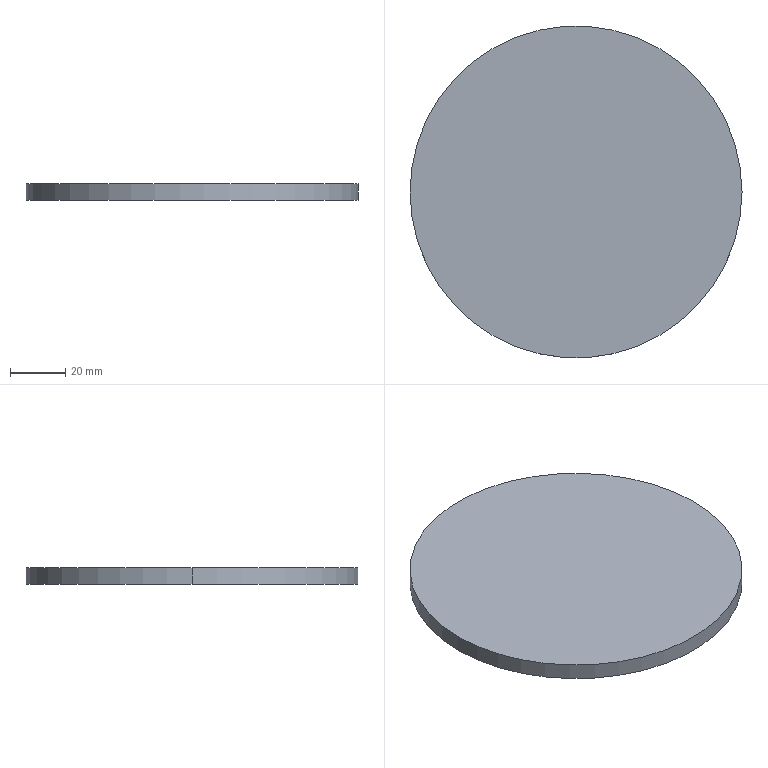Part | SolidWorks | features BaseBody 1 | 1 solid | 4 faces | box 120 x 120 x 6 mm | volume 67858 mm3 | cylinder 2 | plane 2 | commonest cylinder face diameters 120 x2
STEP:
#1=CARTESIAN_POINT('',(-74.453,1729.544,-312.));
#2=VERTEX_POINT('',#1);
#3=CARTESIAN_POINT('',(-194.453,1729.544,-312.));
#4=VERTEX_POINT('',#3);
#5=CARTESIAN_POINT('',(-134.453,1729.544,-312.));
#6=DIRECTION('',(0.,0.,1.));
#7=DIRECTION('',(1.,0.,0.));
#8=AXIS2_PLACEMENT_3D('',#5,#6,#7);
#9=CIRCLE('',#8,60.);
#10=EDGE_CURVE('',#2,#4,#9,.T.);
#11=ORIENTED_EDGE('',*,*,#10,.T.);
#12=CARTESIAN_POINT('',(-194.453,1729.544,-306.));
#13=VERTEX_POINT('',#12);
#14=CARTESIAN_POINT('',(-194.453,1729.544,-312.));
#15=DIRECTION('',(0.,0.,1.));
#16=VECTOR('',#15,1000.);
#17=LINE('',#14,#16);
#18=EDGE_CURVE('',#4,#13,#17,.T.);
#19=ORIENTED_EDGE('',*,*,#18,.T.);
#20=CARTESIAN_POINT('',(-74.453,1729.544,-306.));
#21=VERTEX_POINT('',#20);
#22=CARTESIAN_POINT('',(-134.453,1729.544,-306.));
#23=DIRECTION('',(0.,0.,1.));
#24=DIRECTION('',(1.,0.,0.));
#25=AXIS2_PLACEMENT_3D('',#22,#23,#24);
#26=CIRCLE('',#25,60.);
#27=EDGE_CURVE('',#21,#13,#26,.T.);
#28=ORIENTED_EDGE('',*,*,#27,.F.);
#29=CARTESIAN_POINT('',(-74.453,1729.544,-312.));
#30=DIRECTION('',(0.,0.,1.));
#31=VECTOR('',#30,1000.);
#32=LINE('',#29,#31);
#33=EDGE_CURVE('',#2,#21,#32,.T.);
#34=ORIENTED_EDGE('',*,*,#33,.F.);
#35=EDGE_LOOP('',(#11,#19,#28,#34));
#36=FACE_OUTER_BOUND('',#35,.T.);
#37=CARTESIAN_POINT('',(-134.453,1729.544,-312.));
#38=DIRECTION('',(0.,0.,1.));
#39=DIRECTION('',(1.,0.,0.));
#40=AXIS2_PLACEMENT_3D('',#37,#38,#39);
#41=CYLINDRICAL_SURFACE('',#40,60.);
#42=ADVANCED_FACE('',(#36),#41,.T.);
#43=ORIENTED_EDGE('',*,*,#27,.T.);
#44=CARTESIAN_POINT('',(-134.453,1729.544,-306.));
#45=DIRECTION('',(0.,0.,1.));
#46=DIRECTION('',(1.,0.,0.));
#47=AXIS2_PLACEMENT_3D('',#44,#45,#46);
#48=CIRCLE('',#47,60.);
#49=EDGE_CURVE('',#13,#21,#48,.T.);
#50=ORIENTED_EDGE('',*,*,#49,.T.);
#51=EDGE_LOOP('',(#43,#50));
#52=FACE_OUTER_BOUND('',#51,.T.);
#53=CARTESIAN_POINT('',(-134.453,1729.544,-306.));
#54=DIRECTION('',(0.,0.,1.));
#55=DIRECTION('',(1.,0.,0.));
#56=AXIS2_PLACEMENT_3D('',#53,#54,#55);
#57=PLANE('',#56);
#58=ADVANCED_FACE('',(#52),#57,.T.);
#59=ORIENTED_EDGE('',*,*,#18,.F.);
#60=CARTESIAN_POINT('',(-134.453,1729.544,-312.));
#61=DIRECTION('',(0.,0.,1.));
#62=DIRECTION('',(1.,0.,0.));
#63=AXIS2_PLACEMENT_3D('',#60,#61,#62);
#64=CIRCLE('',#63,60.);
#65=EDGE_CURVE('',#4,#2,#64,.T.);
#66=ORIENTED_EDGE('',*,*,#65,.T.);
#67=ORIENTED_EDGE('',*,*,#33,.T.);
#68=ORIENTED_EDGE('',*,*,#49,.F.);
#69=EDGE_LOOP('',(#59,#66,#67,#68));
#70=FACE_OUTER_BOUND('',#69,.T.);
#71=CARTESIAN_POINT('',(-134.453,1729.544,-312.));
#72=DIRECTION('',(0.,0.,1.));
#73=DIRECTION('',(1.,0.,0.));
#74=AXIS2_PLACEMENT_3D('',#71,#72,#73);
#75=CYLINDRICAL_SURFACE('',#74,60.);
#76=ADVANCED_FACE('',(#70),#75,.T.);
#77=ORIENTED_EDGE('',*,*,#10,.F.);
#78=ORIENTED_EDGE('',*,*,#65,.F.);
#79=EDGE_LOOP('',(#77,#78));
#80=FACE_OUTER_BOUND('',#79,.T.);
#81=CARTESIAN_POINT('',(-134.453,1729.544,-312.));
#82=DIRECTION('',(0.,0.,-1.));
#83=DIRECTION('',(-1.,0.,0.));
#84=AXIS2_PLACEMENT_3D('',#81,#82,#83);
#85=PLANE('',#84);
#86=ADVANCED_FACE('',(#80),#85,.T.);
#87=CLOSED_SHELL('',(#42,#58,#76,#86));
#88=MANIFOLD_SOLID_BREP('',#87);
#89=CARTESIAN_POINT('',(0.,0.,0.));
#90=DIRECTION('',(0.,0.,1.));
#91=DIRECTION('',(1.,0.,0.));
#92=AXIS2_PLACEMENT_3D('',#89,#90,#91);
#93=(LENGTH_UNIT()NAMED_UNIT(*)SI_UNIT(.MILLI.,.METRE.));
#94=UNCERTAINTY_MEASURE_WITH_UNIT(LENGTH_MEASURE(0.00001),#93,'','');
#95=(NAMED_UNIT(*)PLANE_ANGLE_UNIT()SI_UNIT($,.RADIAN.));
#96=(NAMED_UNIT(*)SI_UNIT($,.STERADIAN.)SOLID_ANGLE_UNIT());
#97=(GEOMETRIC_REPRESENTATION_CONTEXT(3)GLOBAL_UNCERTAINTY_ASSIGNED_CONTEXT((#94))GLOBAL_UNIT_ASSIGNED_CONTEXT((#93,#95,#96))REPRESENTATION_CONTEXT('',''));
#98=ADVANCED_BREP_SHAPE_REPRESENTATION('',(#88,#92),#97);